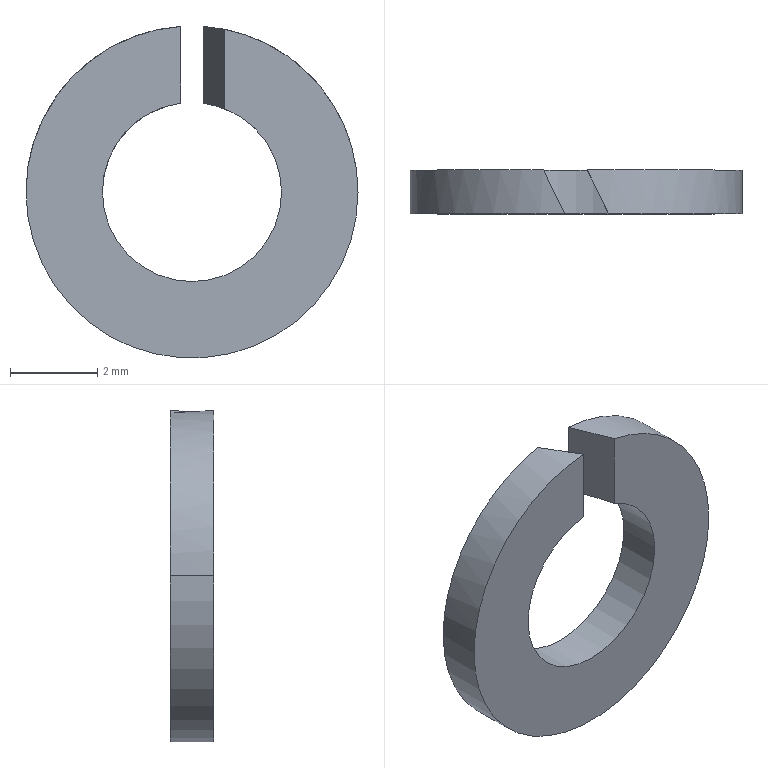Part | STEP file | ZZ24-M4-8 | 1 solid | 10 faces | box 7.6 x 1 x 7.591 mm | volume 30.4 mm3 | cylinder 6 | plane 4 | commonest cylinder face diameters 4.1 x3 7.6 x3
STEP:
#1=CARTESIAN_POINT('',(0.,0.,0.));
#2=DIRECTION('',(0.,0.,1.));
#3=DIRECTION('',(1.,0.,0.));
#4=AXIS2_PLACEMENT_3D('',#1,#2,#3);
#5=CARTESIAN_POINT('',(0.7439,0.,1.91));
#6=VERTEX_POINT('',#5);
#7=CARTESIAN_POINT('',(0.2561,1.,2.034));
#8=VERTEX_POINT('',#7);
#9=CARTESIAN_POINT('',(0.7439,0.,1.91));
#10=CARTESIAN_POINT('',(0.5868,0.3221,1.971));
#11=CARTESIAN_POINT('',(0.4234,0.6571,2.013));
#12=CARTESIAN_POINT('',(0.2561,1.,2.034));
#13=(BOUNDED_CURVE()B_SPLINE_CURVE(3,(#9,#10,#11,#12),.UNSPECIFIED.,.F.,.F.)B_SPLINE_CURVE_WITH_KNOTS((4,4),(1.199,1.446),.PIECEWISE_BEZIER_KNOTS.)CURVE()GEOMETRIC_REPRESENTATION_ITEM()RATIONAL_B_SPLINE_CURVE((1.,0.995,0.995,1.))REPRESENTATION_ITEM(''));
#14=CARTESIAN_POINT('',(0.,1.,0.));
#15=DIRECTION('',(0.,-1.,0.));
#16=DIRECTION('',(-1.,0.,0.001512));
#17=AXIS2_PLACEMENT_3D('',#14,#15,#16);
#18=CYLINDRICAL_SURFACE('',#17,2.05);
#19=CARTESIAN_POINT('',(4.343,1.));
#20=CARTESIAN_POINT('',(4.346,0.9854));
#21=CARTESIAN_POINT('',(4.354,0.9562));
#22=CARTESIAN_POINT('',(4.365,0.9122));
#23=CARTESIAN_POINT('',(4.376,0.868));
#24=CARTESIAN_POINT('',(4.387,0.8236));
#25=CARTESIAN_POINT('',(4.398,0.779));
#26=CARTESIAN_POINT('',(4.41,0.7342));
#27=CARTESIAN_POINT('',(4.421,0.6892));
#28=CARTESIAN_POINT('',(4.432,0.6441));
#29=CARTESIAN_POINT('',(4.443,0.5988));
#30=CARTESIAN_POINT('',(4.454,0.5534));
#31=CARTESIAN_POINT('',(4.466,0.5078));
#32=CARTESIAN_POINT('',(4.477,0.4621));
#33=CARTESIAN_POINT('',(4.488,0.4163));
#34=CARTESIAN_POINT('',(4.499,0.3704));
#35=CARTESIAN_POINT('',(4.51,0.3244));
#36=CARTESIAN_POINT('',(4.522,0.2782));
#37=CARTESIAN_POINT('',(4.533,0.232));
#38=CARTESIAN_POINT('',(4.544,0.1858));
#39=CARTESIAN_POINT('',(4.555,0.1394));
#40=CARTESIAN_POINT('',(4.566,0.09298));
#41=CARTESIAN_POINT('',(4.577,0.04651));
#42=CARTESIAN_POINT('',(4.585,0.01551));
#43=CARTESIAN_POINT('',(4.589,0.));
#44=B_SPLINE_CURVE_WITH_KNOTS('',3,(#19,#20,#21,#22,#23,#24,#25,#26,#27,#28,#29,#30,#31,#32,#33,#34,#35,#36,#37,#38,#39,#40,#41,#42,#43),.UNSPECIFIED.,.F.,.F.,(4,1,1,1,1,1,1,1,1,1,1,1,1,1,1,1,1,1,1,1,1,1,4),(1.199,1.211,1.222,1.233,1.244,1.255,1.267,1.278,1.289,1.3,1.311,1.322,1.334,1.345,1.356,1.367,1.378,1.39,1.401,1.412,1.423,1.434,1.446),.QUASI_UNIFORM_KNOTS.);
#45=(GEOMETRIC_REPRESENTATION_CONTEXT(2)PARAMETRIC_REPRESENTATION_CONTEXT()REPRESENTATION_CONTEXT('',''));
#46=DEFINITIONAL_REPRESENTATION('',(#44),#45);
#47=PCURVE('',#18,#46);
#48=CARTESIAN_POINT('',(0.7439,0.,3.8));
#49=DIRECTION('',(-0.8988,-0.4384,0.));
#50=DIRECTION('',(0.4384,-0.8988,0.));
#51=AXIS2_PLACEMENT_3D('',#48,#49,#50);
#52=PLANE('',#51);
#53=CARTESIAN_POINT('',(0.,-1.89));
#54=CARTESIAN_POINT('',(-0.3583,-1.829));
#55=CARTESIAN_POINT('',(-0.7311,-1.787));
#56=CARTESIAN_POINT('',(-1.113,-1.766));
#57=(BOUNDED_CURVE()B_SPLINE_CURVE(3,(#53,#54,#55,#56),.UNSPECIFIED.,.F.,.F.)B_SPLINE_CURVE_WITH_KNOTS((4,4),(1.199,1.446),.PIECEWISE_BEZIER_KNOTS.)CURVE()GEOMETRIC_REPRESENTATION_ITEM()RATIONAL_B_SPLINE_CURVE((1.,0.995,0.995,1.))REPRESENTATION_ITEM(''));
#58=(GEOMETRIC_REPRESENTATION_CONTEXT(2)PARAMETRIC_REPRESENTATION_CONTEXT()REPRESENTATION_CONTEXT('',''));
#59=DEFINITIONAL_REPRESENTATION('',(#57),#58);
#60=PCURVE('',#52,#59);
#61=SURFACE_CURVE('',#13,(#47,#60),.PCURVE_S1.);
#62=EDGE_CURVE('',#6,#8,#61,.T.);
#63=ORIENTED_EDGE('',*,*,#62,.F.);
#64=CARTESIAN_POINT('',(2.05,0.,-0.0031));
#65=VERTEX_POINT('',#64);
#66=CARTESIAN_POINT('',(0.,0.,0.));
#67=DIRECTION('',(0.,1.,0.));
#68=DIRECTION('',(1.,0.,-0.001512));
#69=AXIS2_PLACEMENT_3D('',#66,#67,#68);
#70=CIRCLE('',#69,2.05);
#71=CARTESIAN_POINT('',(9.425,1.));
#72=DIRECTION('',(-1.,0.));
#73=VECTOR('',#72,1.);
#74=LINE('',#71,#73);
#75=(GEOMETRIC_REPRESENTATION_CONTEXT(2)PARAMETRIC_REPRESENTATION_CONTEXT()REPRESENTATION_CONTEXT('',''));
#76=DEFINITIONAL_REPRESENTATION('',(#74),#75);
#77=PCURVE('',#18,#76);
#78=CARTESIAN_POINT('',(0.,0.,0.));
#79=DIRECTION('',(0.,-1.,0.));
#80=DIRECTION('',(-1.,0.,0.001512));
#81=AXIS2_PLACEMENT_3D('',#78,#79,#80);
#82=PLANE('',#81);
#83=CARTESIAN_POINT('',(-2.05,0.));
#84=CARTESIAN_POINT('',(-2.05,3.551));
#85=CARTESIAN_POINT('',(1.025,1.775));
#86=CARTESIAN_POINT('',(4.1,0.));
#87=CARTESIAN_POINT('',(1.025,-1.775));
#88=CARTESIAN_POINT('',(-2.05,-3.551));
#89=CARTESIAN_POINT('',(-2.05,0.));
#90=(BOUNDED_CURVE()B_SPLINE_CURVE(2,(#83,#84,#85,#86,#87,#88,#89),.UNSPECIFIED.,.T.,.F.)B_SPLINE_CURVE_WITH_KNOTS((1,2,2,2,2,1),(-2.094,0.,2.094,4.189,6.283,8.378),.UNSPECIFIED.)CURVE()GEOMETRIC_REPRESENTATION_ITEM()RATIONAL_B_SPLINE_CURVE((1.,0.5,1.,0.5,1.,0.5,1.))REPRESENTATION_ITEM(''));
#91=(GEOMETRIC_REPRESENTATION_CONTEXT(2)PARAMETRIC_REPRESENTATION_CONTEXT()REPRESENTATION_CONTEXT('',''));
#92=DEFINITIONAL_REPRESENTATION('',(#90),#91);
#93=PCURVE('',#82,#92);
#94=SURFACE_CURVE('',#70,(#77,#93),.PCURVE_S1.);
#95=EDGE_CURVE('',#6,#65,#94,.T.);
#96=ORIENTED_EDGE('',*,*,#95,.T.);
#97=CARTESIAN_POINT('',(2.05,1.,-0.0031));
#98=VERTEX_POINT('',#97);
#99=CARTESIAN_POINT('',(2.05,1.,-0.0031));
#100=DIRECTION('',(0.,-1.,0.));
#101=VECTOR('',#100,1.);
#102=LINE('',#99,#101);
#103=CARTESIAN_POINT('',(3.142,0.));
#104=DIRECTION('',(0.,1.));
#105=VECTOR('',#104,1.);
#106=LINE('',#103,#105);
#107=(GEOMETRIC_REPRESENTATION_CONTEXT(2)PARAMETRIC_REPRESENTATION_CONTEXT()REPRESENTATION_CONTEXT('',''));
#108=DEFINITIONAL_REPRESENTATION('',(#106),#107);
#109=PCURVE('',#18,#108);
#110=CARTESIAN_POINT('',(0.,1.,0.));
#111=DIRECTION('',(0.,-1.,0.));
#112=DIRECTION('',(-1.,0.,0.001512));
#113=AXIS2_PLACEMENT_3D('',#110,#111,#112);
#114=CYLINDRICAL_SURFACE('',#113,2.05);
#115=CARTESIAN_POINT('',(3.142,0.));
#116=DIRECTION('',(0.,1.));
#117=VECTOR('',#116,1.);
#118=LINE('',#115,#117);
#119=(GEOMETRIC_REPRESENTATION_CONTEXT(2)PARAMETRIC_REPRESENTATION_CONTEXT()REPRESENTATION_CONTEXT('',''));
#120=DEFINITIONAL_REPRESENTATION('',(#118),#119);
#121=PCURVE('',#114,#120);
#122=SURFACE_CURVE('',#102,(#109,#121),.PCURVE_S1.);
#123=EDGE_CURVE('',#98,#65,#122,.T.);
#124=ORIENTED_EDGE('',*,*,#123,.F.);
#125=CARTESIAN_POINT('',(0.,1.,0.));
#126=DIRECTION('',(0.,-1.,0.));
#127=DIRECTION('',(-1.,0.,0.001512));
#128=AXIS2_PLACEMENT_3D('',#125,#126,#127);
#129=CIRCLE('',#128,2.05);
#130=CARTESIAN_POINT('',(0.,0.));
#131=DIRECTION('',(1.,0.));
#132=VECTOR('',#131,1.);
#133=LINE('',#130,#132);
#134=(GEOMETRIC_REPRESENTATION_CONTEXT(2)PARAMETRIC_REPRESENTATION_CONTEXT()REPRESENTATION_CONTEXT('',''));
#135=DEFINITIONAL_REPRESENTATION('',(#133),#134);
#136=PCURVE('',#18,#135);
#137=CARTESIAN_POINT('',(0.,1.,0.));
#138=DIRECTION('',(0.,1.,0.));
#139=DIRECTION('',(1.,0.,-0.001512));
#140=AXIS2_PLACEMENT_3D('',#137,#138,#139);
#141=PLANE('',#140);
#142=CARTESIAN_POINT('',(-2.05,0.));
#143=CARTESIAN_POINT('',(-2.05,3.551));
#144=CARTESIAN_POINT('',(1.025,1.775));
#145=CARTESIAN_POINT('',(4.1,0.));
#146=CARTESIAN_POINT('',(1.025,-1.775));
#147=CARTESIAN_POINT('',(-2.05,-3.551));
#148=CARTESIAN_POINT('',(-2.05,0.));
#149=(BOUNDED_CURVE()B_SPLINE_CURVE(2,(#142,#143,#144,#145,#146,#147,#148),.UNSPECIFIED.,.T.,.F.)B_SPLINE_CURVE_WITH_KNOTS((1,2,2,2,2,1),(-2.094,0.,2.094,4.189,6.283,8.378),.UNSPECIFIED.)CURVE()GEOMETRIC_REPRESENTATION_ITEM()RATIONAL_B_SPLINE_CURVE((1.,0.5,1.,0.5,1.,0.5,1.))REPRESENTATION_ITEM(''));
#150=(GEOMETRIC_REPRESENTATION_CONTEXT(2)PARAMETRIC_REPRESENTATION_CONTEXT()REPRESENTATION_CONTEXT('',''));
#151=DEFINITIONAL_REPRESENTATION('',(#149),#150);
#152=PCURVE('',#141,#151);
#153=SURFACE_CURVE('',#129,(#136,#152),.PCURVE_S1.);
#154=EDGE_CURVE('',#98,#8,#153,.T.);
#155=ORIENTED_EDGE('',*,*,#154,.T.);
#156=EDGE_LOOP('',(#63,#96,#124,#155));
#157=FACE_BOUND('',#156,.F.);
#158=ADVANCED_FACE('',(#157),#18,.F.);
#159=CARTESIAN_POINT('',(-2.05,0.,0.0031));
#160=VERTEX_POINT('',#159);
#161=CARTESIAN_POINT('',(0.,0.,0.));
#162=DIRECTION('',(0.,1.,0.));
#163=DIRECTION('',(1.,0.,-0.001512));
#164=AXIS2_PLACEMENT_3D('',#161,#162,#163);
#165=CIRCLE('',#164,2.05);
#166=CARTESIAN_POINT('',(3.142,1.));
#167=DIRECTION('',(-1.,0.));
#168=VECTOR('',#167,1.);
#169=LINE('',#166,#168);
#170=(GEOMETRIC_REPRESENTATION_CONTEXT(2)PARAMETRIC_REPRESENTATION_CONTEXT()REPRESENTATION_CONTEXT('',''));
#171=DEFINITIONAL_REPRESENTATION('',(#169),#170);
#172=PCURVE('',#114,#171);
#173=CARTESIAN_POINT('',(-2.05,0.));
#174=CARTESIAN_POINT('',(-2.05,3.551));
#175=CARTESIAN_POINT('',(1.025,1.775));
#176=CARTESIAN_POINT('',(4.1,0.));
#177=CARTESIAN_POINT('',(1.025,-1.775));
#178=CARTESIAN_POINT('',(-2.05,-3.551));
#179=CARTESIAN_POINT('',(-2.05,0.));
#180=(BOUNDED_CURVE()B_SPLINE_CURVE(2,(#173,#174,#175,#176,#177,#178,#179),.UNSPECIFIED.,.T.,.F.)B_SPLINE_CURVE_WITH_KNOTS((1,2,2,2,2,1),(-2.094,0.,2.094,4.189,6.283,8.378),.UNSPECIFIED.)CURVE()GEOMETRIC_REPRESENTATION_ITEM()RATIONAL_B_SPLINE_CURVE((1.,0.5,1.,0.5,1.,0.5,1.))REPRESENTATION_ITEM(''));
#181=(GEOMETRIC_REPRESENTATION_CONTEXT(2)PARAMETRIC_REPRESENTATION_CONTEXT()REPRESENTATION_CONTEXT('',''));
#182=DEFINITIONAL_REPRESENTATION('',(#180),#181);
#183=PCURVE('',#82,#182);
#184=SURFACE_CURVE('',#165,(#172,#183),.PCURVE_S1.);
#185=EDGE_CURVE('',#65,#160,#184,.T.);
#186=ORIENTED_EDGE('',*,*,#185,.T.);
#187=CARTESIAN_POINT('',(-2.05,1.,0.0031));
#188=VERTEX_POINT('',#187);
#189=CARTESIAN_POINT('',(-2.05,1.,0.0031));
#190=DIRECTION('',(0.,-1.,0.));
#191=VECTOR('',#190,1.);
#192=LINE('',#189,#191);
#193=CARTESIAN_POINT('',(0.,0.));
#194=DIRECTION('',(0.,1.));
#195=VECTOR('',#194,1.);
#196=LINE('',#193,#195);
#197=(GEOMETRIC_REPRESENTATION_CONTEXT(2)PARAMETRIC_REPRESENTATION_CONTEXT()REPRESENTATION_CONTEXT('',''));
#198=DEFINITIONAL_REPRESENTATION('',(#196),#197);
#199=PCURVE('',#114,#198);
#200=CARTESIAN_POINT('',(0.,1.,0.));
#201=DIRECTION('',(0.,-1.,0.));
#202=DIRECTION('',(-1.,0.,0.001512));
#203=AXIS2_PLACEMENT_3D('',#200,#201,#202);
#204=CYLINDRICAL_SURFACE('',#203,2.05);
#205=CARTESIAN_POINT('',(6.283,0.));
#206=DIRECTION('',(0.,1.));
#207=VECTOR('',#206,1.);
#208=LINE('',#205,#207);
#209=(GEOMETRIC_REPRESENTATION_CONTEXT(2)PARAMETRIC_REPRESENTATION_CONTEXT()REPRESENTATION_CONTEXT('',''));
#210=DEFINITIONAL_REPRESENTATION('',(#208),#209);
#211=PCURVE('',#204,#210);
#212=SURFACE_CURVE('',#192,(#199,#211),.PCURVE_S1.);
#213=EDGE_CURVE('',#188,#160,#212,.T.);
#214=ORIENTED_EDGE('',*,*,#213,.F.);
#215=CARTESIAN_POINT('',(0.,1.,0.));
#216=DIRECTION('',(0.,-1.,0.));
#217=DIRECTION('',(-1.,0.,0.001512));
#218=AXIS2_PLACEMENT_3D('',#215,#216,#217);
#219=CIRCLE('',#218,2.05);
#220=CARTESIAN_POINT('',(0.,0.));
#221=DIRECTION('',(1.,0.));
#222=VECTOR('',#221,1.);
#223=LINE('',#220,#222);
#224=(GEOMETRIC_REPRESENTATION_CONTEXT(2)PARAMETRIC_REPRESENTATION_CONTEXT()REPRESENTATION_CONTEXT('',''));
#225=DEFINITIONAL_REPRESENTATION('',(#223),#224);
#226=PCURVE('',#114,#225);
#227=CARTESIAN_POINT('',(-2.05,0.));
#228=CARTESIAN_POINT('',(-2.05,3.551));
#229=CARTESIAN_POINT('',(1.025,1.775));
#230=CARTESIAN_POINT('',(4.1,0.));
#231=CARTESIAN_POINT('',(1.025,-1.775));
#232=CARTESIAN_POINT('',(-2.05,-3.551));
#233=CARTESIAN_POINT('',(-2.05,0.));
#234=(BOUNDED_CURVE()B_SPLINE_CURVE(2,(#227,#228,#229,#230,#231,#232,#233),.UNSPECIFIED.,.T.,.F.)B_SPLINE_CURVE_WITH_KNOTS((1,2,2,2,2,1),(-2.094,0.,2.094,4.189,6.283,8.378),.UNSPECIFIED.)CURVE()GEOMETRIC_REPRESENTATION_ITEM()RATIONAL_B_SPLINE_CURVE((1.,0.5,1.,0.5,1.,0.5,1.))REPRESENTATION_ITEM(''));
#235=(GEOMETRIC_REPRESENTATION_CONTEXT(2)PARAMETRIC_REPRESENTATION_CONTEXT()REPRESENTATION_CONTEXT('',''));
#236=DEFINITIONAL_REPRESENTATION('',(#234),#235);
#237=PCURVE('',#141,#236);
#238=SURFACE_CURVE('',#219,(#226,#237),.PCURVE_S1.);
#239=EDGE_CURVE('',#188,#98,#238,.T.);
#240=ORIENTED_EDGE('',*,*,#239,.T.);
#241=ORIENTED_EDGE('',*,*,#123,.T.);
#242=EDGE_LOOP('',(#186,#214,#240,#241));
#243=FACE_BOUND('',#242,.F.);
#244=ADVANCED_FACE('',(#243),#114,.F.);
#245=CARTESIAN_POINT('',(-3.8,1.,0.005747));
#246=VERTEX_POINT('',#245);
#247=CARTESIAN_POINT('',(3.8,1.,-0.005747));
#248=VERTEX_POINT('',#247);
#249=CARTESIAN_POINT('',(0.,1.,0.));
#250=DIRECTION('',(0.,-1.,0.));
#251=DIRECTION('',(-1.,0.,0.001512));
#252=AXIS2_PLACEMENT_3D('',#249,#250,#251);
#253=CIRCLE('',#252,3.8);
#254=CARTESIAN_POINT('',(0.,1.,0.));
#255=DIRECTION('',(0.,-1.,0.));
#256=DIRECTION('',(-1.,0.,0.001512));
#257=AXIS2_PLACEMENT_3D('',#254,#255,#256);
#258=CYLINDRICAL_SURFACE('',#257,3.8);
#259=CARTESIAN_POINT('',(0.,0.));
#260=DIRECTION('',(1.,0.));
#261=VECTOR('',#260,1.);
#262=LINE('',#259,#261);
#263=(GEOMETRIC_REPRESENTATION_CONTEXT(2)PARAMETRIC_REPRESENTATION_CONTEXT()REPRESENTATION_CONTEXT('',''));
#264=DEFINITIONAL_REPRESENTATION('',(#262),#263);
#265=PCURVE('',#258,#264);
#266=CARTESIAN_POINT('',(-3.8,0.));
#267=CARTESIAN_POINT('',(-3.8,6.582));
#268=CARTESIAN_POINT('',(1.9,3.291));
#269=CARTESIAN_POINT('',(7.6,0.));
#270=CARTESIAN_POINT('',(1.9,-3.291));
#271=CARTESIAN_POINT('',(-3.8,-6.582));
#272=CARTESIAN_POINT('',(-3.8,0.));
#273=(BOUNDED_CURVE()B_SPLINE_CURVE(2,(#266,#267,#268,#269,#270,#271,#272),.UNSPECIFIED.,.T.,.F.)B_SPLINE_CURVE_WITH_KNOTS((1,2,2,2,2,1),(-2.094,0.,2.094,4.189,6.283,8.378),.UNSPECIFIED.)CURVE()GEOMETRIC_REPRESENTATION_ITEM()RATIONAL_B_SPLINE_CURVE((1.,0.5,1.,0.5,1.,0.5,1.))REPRESENTATION_ITEM(''));
#274=(GEOMETRIC_REPRESENTATION_CONTEXT(2)PARAMETRIC_REPRESENTATION_CONTEXT()REPRESENTATION_CONTEXT('',''));
#275=DEFINITIONAL_REPRESENTATION('',(#273),#274);
#276=PCURVE('',#141,#275);
#277=SURFACE_CURVE('',#253,(#265,#276),.PCURVE_S1.);
#278=EDGE_CURVE('',#246,#248,#277,.T.);
#279=ORIENTED_EDGE('',*,*,#278,.T.);
#280=CARTESIAN_POINT('',(3.8,0.,-0.005747));
#281=VERTEX_POINT('',#280);
#282=CARTESIAN_POINT('',(3.8,1.,-0.005747));
#283=DIRECTION('',(0.,-1.,0.));
#284=VECTOR('',#283,1.);
#285=LINE('',#282,#284);
#286=CARTESIAN_POINT('',(3.142,0.));
#287=DIRECTION('',(0.,1.));
#288=VECTOR('',#287,1.);
#289=LINE('',#286,#288);
#290=(GEOMETRIC_REPRESENTATION_CONTEXT(2)PARAMETRIC_REPRESENTATION_CONTEXT()REPRESENTATION_CONTEXT('',''));
#291=DEFINITIONAL_REPRESENTATION('',(#289),#290);
#292=PCURVE('',#258,#291);
#293=CARTESIAN_POINT('',(0.,1.,0.));
#294=DIRECTION('',(0.,-1.,0.));
#295=DIRECTION('',(-1.,0.,0.001512));
#296=AXIS2_PLACEMENT_3D('',#293,#294,#295);
#297=CYLINDRICAL_SURFACE('',#296,3.8);
#298=CARTESIAN_POINT('',(3.142,0.));
#299=DIRECTION('',(0.,1.));
#300=VECTOR('',#299,1.);
#301=LINE('',#298,#300);
#302=(GEOMETRIC_REPRESENTATION_CONTEXT(2)PARAMETRIC_REPRESENTATION_CONTEXT()REPRESENTATION_CONTEXT('',''));
#303=DEFINITIONAL_REPRESENTATION('',(#301),#302);
#304=PCURVE('',#297,#303);
#305=SURFACE_CURVE('',#285,(#292,#304),.PCURVE_S1.);
#306=EDGE_CURVE('',#248,#281,#305,.T.);
#307=ORIENTED_EDGE('',*,*,#306,.T.);
#308=CARTESIAN_POINT('',(-3.8,0.,0.005747));
#309=VERTEX_POINT('',#308);
#310=CARTESIAN_POINT('',(0.,0.,0.));
#311=DIRECTION('',(0.,1.,0.));
#312=DIRECTION('',(1.,0.,-0.001512));
#313=AXIS2_PLACEMENT_3D('',#310,#311,#312);
#314=CIRCLE('',#313,3.8);
#315=CARTESIAN_POINT('',(3.142,1.));
#316=DIRECTION('',(-1.,0.));
#317=VECTOR('',#316,1.);
#318=LINE('',#315,#317);
#319=(GEOMETRIC_REPRESENTATION_CONTEXT(2)PARAMETRIC_REPRESENTATION_CONTEXT()REPRESENTATION_CONTEXT('',''));
#320=DEFINITIONAL_REPRESENTATION('',(#318),#319);
#321=PCURVE('',#258,#320);
#322=CARTESIAN_POINT('',(-3.8,0.));
#323=CARTESIAN_POINT('',(-3.8,6.582));
#324=CARTESIAN_POINT('',(1.9,3.291));
#325=CARTESIAN_POINT('',(7.6,0.));
#326=CARTESIAN_POINT('',(1.9,-3.291));
#327=CARTESIAN_POINT('',(-3.8,-6.582));
#328=CARTESIAN_POINT('',(-3.8,0.));
#329=(BOUNDED_CURVE()B_SPLINE_CURVE(2,(#322,#323,#324,#325,#326,#327,#328),.UNSPECIFIED.,.T.,.F.)B_SPLINE_CURVE_WITH_KNOTS((1,2,2,2,2,1),(-2.094,0.,2.094,4.189,6.283,8.378),.UNSPECIFIED.)CURVE()GEOMETRIC_REPRESENTATION_ITEM()RATIONAL_B_SPLINE_CURVE((1.,0.5,1.,0.5,1.,0.5,1.))REPRESENTATION_ITEM(''));
#330=(GEOMETRIC_REPRESENTATION_CONTEXT(2)PARAMETRIC_REPRESENTATION_CONTEXT()REPRESENTATION_CONTEXT('',''));
#331=DEFINITIONAL_REPRESENTATION('',(#329),#330);
#332=PCURVE('',#82,#331);
#333=SURFACE_CURVE('',#314,(#321,#332),.PCURVE_S1.);
#334=EDGE_CURVE('',#281,#309,#333,.T.);
#335=ORIENTED_EDGE('',*,*,#334,.T.);
#336=CARTESIAN_POINT('',(-3.8,1.,0.005747));
#337=DIRECTION('',(0.,-1.,0.));
#338=VECTOR('',#337,1.);
#339=LINE('',#336,#338);
#340=CARTESIAN_POINT('',(0.,0.));
#341=DIRECTION('',(0.,1.));
#342=VECTOR('',#341,1.);
#343=LINE('',#340,#342);
#344=(GEOMETRIC_REPRESENTATION_CONTEXT(2)PARAMETRIC_REPRESENTATION_CONTEXT()REPRESENTATION_CONTEXT('',''));
#345=DEFINITIONAL_REPRESENTATION('',(#343),#344);
#346=PCURVE('',#258,#345);
#347=CARTESIAN_POINT('',(0.,1.,0.));
#348=DIRECTION('',(0.,-1.,0.));
#349=DIRECTION('',(-1.,0.,0.001512));
#350=AXIS2_PLACEMENT_3D('',#347,#348,#349);
#351=CYLINDRICAL_SURFACE('',#350,3.8);
#352=CARTESIAN_POINT('',(6.283,0.));
#353=DIRECTION('',(0.,1.));
#354=VECTOR('',#353,1.);
#355=LINE('',#352,#354);
#356=(GEOMETRIC_REPRESENTATION_CONTEXT(2)PARAMETRIC_REPRESENTATION_CONTEXT()REPRESENTATION_CONTEXT('',''));
#357=DEFINITIONAL_REPRESENTATION('',(#355),#356);
#358=PCURVE('',#351,#357);
#359=SURFACE_CURVE('',#339,(#346,#358),.PCURVE_S1.);
#360=EDGE_CURVE('',#246,#309,#359,.T.);
#361=ORIENTED_EDGE('',*,*,#360,.F.);
#362=EDGE_LOOP('',(#279,#307,#335,#361));
#363=FACE_BOUND('',#362,.T.);
#364=ADVANCED_FACE('',(#363),#258,.T.);
#365=CARTESIAN_POINT('',(-0.7439,1.,3.726));
#366=VERTEX_POINT('',#365);
#367=CARTESIAN_POINT('',(0.,1.,0.));
#368=DIRECTION('',(0.,-1.,0.));
#369=DIRECTION('',(-1.,0.,0.001512));
#370=AXIS2_PLACEMENT_3D('',#367,#368,#369);
#371=CIRCLE('',#370,3.8);
#372=CARTESIAN_POINT('',(0.,0.));
#373=DIRECTION('',(1.,0.));
#374=VECTOR('',#373,1.);
#375=LINE('',#372,#374);
#376=(GEOMETRIC_REPRESENTATION_CONTEXT(2)PARAMETRIC_REPRESENTATION_CONTEXT()REPRESENTATION_CONTEXT('',''));
#377=DEFINITIONAL_REPRESENTATION('',(#375),#376);
#378=PCURVE('',#351,#377);
#379=CARTESIAN_POINT('',(-3.8,0.));
#380=CARTESIAN_POINT('',(-3.8,6.582));
#381=CARTESIAN_POINT('',(1.9,3.291));
#382=CARTESIAN_POINT('',(7.6,0.));
#383=CARTESIAN_POINT('',(1.9,-3.291));
#384=CARTESIAN_POINT('',(-3.8,-6.582));
#385=CARTESIAN_POINT('',(-3.8,0.));
#386=(BOUNDED_CURVE()B_SPLINE_CURVE(2,(#379,#380,#381,#382,#383,#384,#385),.UNSPECIFIED.,.T.,.F.)B_SPLINE_CURVE_WITH_KNOTS((1,2,2,2,2,1),(-2.094,0.,2.094,4.189,6.283,8.378),.UNSPECIFIED.)CURVE()GEOMETRIC_REPRESENTATION_ITEM()RATIONAL_B_SPLINE_CURVE((1.,0.5,1.,0.5,1.,0.5,1.))REPRESENTATION_ITEM(''));
#387=(GEOMETRIC_REPRESENTATION_CONTEXT(2)PARAMETRIC_REPRESENTATION_CONTEXT()REPRESENTATION_CONTEXT('',''));
#388=DEFINITIONAL_REPRESENTATION('',(#386),#387);
#389=PCURVE('',#141,#388);
#390=SURFACE_CURVE('',#371,(#378,#389),.PCURVE_S1.);
#391=EDGE_CURVE('',#366,#246,#390,.T.);
#392=ORIENTED_EDGE('',*,*,#391,.T.);
#393=ORIENTED_EDGE('',*,*,#360,.T.);
#394=CARTESIAN_POINT('',(-0.2561,0.,3.791));
#395=VERTEX_POINT('',#394);
#396=CARTESIAN_POINT('',(0.,0.,0.));
#397=DIRECTION('',(0.,1.,0.));
#398=DIRECTION('',(1.,0.,-0.001512));
#399=AXIS2_PLACEMENT_3D('',#396,#397,#398);
#400=CIRCLE('',#399,3.8);
#401=CARTESIAN_POINT('',(9.425,1.));
#402=DIRECTION('',(-1.,0.));
#403=VECTOR('',#402,1.);
#404=LINE('',#401,#403);
#405=(GEOMETRIC_REPRESENTATION_CONTEXT(2)PARAMETRIC_REPRESENTATION_CONTEXT()REPRESENTATION_CONTEXT('',''));
#406=DEFINITIONAL_REPRESENTATION('',(#404),#405);
#407=PCURVE('',#351,#406);
#408=CARTESIAN_POINT('',(-3.8,0.));
#409=CARTESIAN_POINT('',(-3.8,6.582));
#410=CARTESIAN_POINT('',(1.9,3.291));
#411=CARTESIAN_POINT('',(7.6,0.));
#412=CARTESIAN_POINT('',(1.9,-3.291));
#413=CARTESIAN_POINT('',(-3.8,-6.582));
#414=CARTESIAN_POINT('',(-3.8,0.));
#415=(BOUNDED_CURVE()B_SPLINE_CURVE(2,(#408,#409,#410,#411,#412,#413,#414),.UNSPECIFIED.,.T.,.F.)B_SPLINE_CURVE_WITH_KNOTS((1,2,2,2,2,1),(-2.094,0.,2.094,4.189,6.283,8.378),.UNSPECIFIED.)CURVE()GEOMETRIC_REPRESENTATION_ITEM()RATIONAL_B_SPLINE_CURVE((1.,0.5,1.,0.5,1.,0.5,1.))REPRESENTATION_ITEM(''));
#416=(GEOMETRIC_REPRESENTATION_CONTEXT(2)PARAMETRIC_REPRESENTATION_CONTEXT()REPRESENTATION_CONTEXT('',''));
#417=DEFINITIONAL_REPRESENTATION('',(#415),#416);
#418=PCURVE('',#82,#417);
#419=SURFACE_CURVE('',#400,(#407,#418),.PCURVE_S1.);
#420=EDGE_CURVE('',#309,#395,#419,.T.);
#421=ORIENTED_EDGE('',*,*,#420,.T.);
#422=CARTESIAN_POINT('',(-0.2561,0.,3.791));
#423=CARTESIAN_POINT('',(-0.42,0.336,3.78));
#424=CARTESIAN_POINT('',(-0.5828,0.6698,3.759));
#425=CARTESIAN_POINT('',(-0.7439,1.,3.726));
#426=(BOUNDED_CURVE()B_SPLINE_CURVE(3,(#422,#423,#424,#425),.UNSPECIFIED.,.F.,.F.)B_SPLINE_CURVE_WITH_KNOTS((4,4),(1.638,1.768),.PIECEWISE_BEZIER_KNOTS.)CURVE()GEOMETRIC_REPRESENTATION_ITEM()RATIONAL_B_SPLINE_CURVE((1.,0.9986,0.9986,1.))REPRESENTATION_ITEM(''));
#427=CARTESIAN_POINT('',(4.781,1.));
#428=CARTESIAN_POINT('',(4.783,0.9847));
#429=CARTESIAN_POINT('',(4.787,0.9543));
#430=CARTESIAN_POINT('',(4.793,0.9085));
#431=CARTESIAN_POINT('',(4.799,0.8628));
#432=CARTESIAN_POINT('',(4.805,0.8171));
#433=CARTESIAN_POINT('',(4.811,0.7714));
#434=CARTESIAN_POINT('',(4.817,0.7257));
#435=CARTESIAN_POINT('',(4.823,0.6801));
#436=CARTESIAN_POINT('',(4.828,0.6345));
#437=CARTESIAN_POINT('',(4.834,0.5889));
#438=CARTESIAN_POINT('',(4.84,0.5434));
#439=CARTESIAN_POINT('',(4.846,0.4978));
#440=CARTESIAN_POINT('',(4.852,0.4524));
#441=CARTESIAN_POINT('',(4.858,0.4069));
#442=CARTESIAN_POINT('',(4.864,0.3615));
#443=CARTESIAN_POINT('',(4.87,0.3161));
#444=CARTESIAN_POINT('',(4.876,0.2708));
#445=CARTESIAN_POINT('',(4.881,0.2255));
#446=CARTESIAN_POINT('',(4.887,0.1803));
#447=CARTESIAN_POINT('',(4.893,0.1352));
#448=CARTESIAN_POINT('',(4.899,0.09005));
#449=CARTESIAN_POINT('',(4.905,0.04499));
#450=CARTESIAN_POINT('',(4.909,0.01499));
#451=CARTESIAN_POINT('',(4.911,0.));
#452=B_SPLINE_CURVE_WITH_KNOTS('',3,(#427,#428,#429,#430,#431,#432,#433,#434,#435,#436,#437,#438,#439,#440,#441,#442,#443,#444,#445,#446,#447,#448,#449,#450,#451),.UNSPECIFIED.,.F.,.F.,(4,1,1,1,1,1,1,1,1,1,1,1,1,1,1,1,1,1,1,1,1,1,4),(1.638,1.644,1.65,1.656,1.662,1.668,1.674,1.679,1.685,1.691,1.697,1.703,1.709,1.715,1.721,1.727,1.732,1.738,1.744,1.75,1.756,1.762,1.768),.QUASI_UNIFORM_KNOTS.);
#453=(GEOMETRIC_REPRESENTATION_CONTEXT(2)PARAMETRIC_REPRESENTATION_CONTEXT()REPRESENTATION_CONTEXT('',''));
#454=DEFINITIONAL_REPRESENTATION('',(#452),#453);
#455=PCURVE('',#351,#454);
#456=CARTESIAN_POINT('',(-0.7439,1.,3.8));
#457=DIRECTION('',(0.8988,0.4384,0.));
#458=DIRECTION('',(-0.4384,0.8988,0.));
#459=AXIS2_PLACEMENT_3D('',#456,#457,#458);
#460=PLANE('',#459);
#461=CARTESIAN_POINT('',(-1.113,-0.008642));
#462=CARTESIAN_POINT('',(-0.7388,-0.01971));
#463=CARTESIAN_POINT('',(-0.3674,-0.04137));
#464=CARTESIAN_POINT('',(0.,-0.07352));
#465=(BOUNDED_CURVE()B_SPLINE_CURVE(3,(#461,#462,#463,#464),.UNSPECIFIED.,.F.,.F.)B_SPLINE_CURVE_WITH_KNOTS((4,4),(1.638,1.768),.PIECEWISE_BEZIER_KNOTS.)CURVE()GEOMETRIC_REPRESENTATION_ITEM()RATIONAL_B_SPLINE_CURVE((1.,0.9986,0.9986,1.))REPRESENTATION_ITEM(''));
#466=(GEOMETRIC_REPRESENTATION_CONTEXT(2)PARAMETRIC_REPRESENTATION_CONTEXT()REPRESENTATION_CONTEXT('',''));
#467=DEFINITIONAL_REPRESENTATION('',(#465),#466);
#468=PCURVE('',#460,#467);
#469=SURFACE_CURVE('',#426,(#455,#468),.PCURVE_S1.);
#470=EDGE_CURVE('',#395,#366,#469,.T.);
#471=ORIENTED_EDGE('',*,*,#470,.T.);
#472=EDGE_LOOP('',(#392,#393,#421,#471));
#473=FACE_BOUND('',#472,.T.);
#474=ADVANCED_FACE('',(#473),#351,.T.);
#475=CARTESIAN_POINT('',(-0.2561,0.,2.034));
#476=VERTEX_POINT('',#475);
#477=CARTESIAN_POINT('',(-0.2561,0.,3.8));
#478=DIRECTION('',(0.,0.,-1.));
#479=VECTOR('',#478,1.);
#480=LINE('',#477,#479);
#481=CARTESIAN_POINT('',(0.2619,-3.8));
#482=DIRECTION('',(-0.001512,1.));
#483=VECTOR('',#482,1.);
#484=LINE('',#481,#483);
#485=(GEOMETRIC_REPRESENTATION_CONTEXT(2)PARAMETRIC_REPRESENTATION_CONTEXT()REPRESENTATION_CONTEXT('',''));
#486=DEFINITIONAL_REPRESENTATION('',(#484),#485);
#487=PCURVE('',#82,#486);
#488=CARTESIAN_POINT('',(-1.113,0.));
#489=DIRECTION('',(0.,-1.));
#490=VECTOR('',#489,1.);
#491=LINE('',#488,#490);
#492=(GEOMETRIC_REPRESENTATION_CONTEXT(2)PARAMETRIC_REPRESENTATION_CONTEXT()REPRESENTATION_CONTEXT('',''));
#493=DEFINITIONAL_REPRESENTATION('',(#491),#492);
#494=PCURVE('',#460,#493);
#495=SURFACE_CURVE('',#480,(#487,#494),.PCURVE_S1.);
#496=EDGE_CURVE('',#395,#476,#495,.T.);
#497=ORIENTED_EDGE('',*,*,#496,.F.);
#498=ORIENTED_EDGE('',*,*,#420,.F.);
#499=ORIENTED_EDGE('',*,*,#334,.F.);
#500=CARTESIAN_POINT('',(0.7439,0.,3.726));
#501=VERTEX_POINT('',#500);
#502=CARTESIAN_POINT('',(0.,0.,0.));
#503=DIRECTION('',(0.,1.,0.));
#504=DIRECTION('',(1.,0.,-0.001512));
#505=AXIS2_PLACEMENT_3D('',#502,#503,#504);
#506=CIRCLE('',#505,3.8);
#507=CARTESIAN_POINT('',(-3.8,0.));
#508=CARTESIAN_POINT('',(-3.8,6.582));
#509=CARTESIAN_POINT('',(1.9,3.291));
#510=CARTESIAN_POINT('',(7.6,0.));
#511=CARTESIAN_POINT('',(1.9,-3.291));
#512=CARTESIAN_POINT('',(-3.8,-6.582));
#513=CARTESIAN_POINT('',(-3.8,0.));
#514=(BOUNDED_CURVE()B_SPLINE_CURVE(2,(#507,#508,#509,#510,#511,#512,#513),.UNSPECIFIED.,.T.,.F.)B_SPLINE_CURVE_WITH_KNOTS((1,2,2,2,2,1),(-2.094,0.,2.094,4.189,6.283,8.378),.UNSPECIFIED.)CURVE()GEOMETRIC_REPRESENTATION_ITEM()RATIONAL_B_SPLINE_CURVE((1.,0.5,1.,0.5,1.,0.5,1.))REPRESENTATION_ITEM(''));
#515=(GEOMETRIC_REPRESENTATION_CONTEXT(2)PARAMETRIC_REPRESENTATION_CONTEXT()REPRESENTATION_CONTEXT('',''));
#516=DEFINITIONAL_REPRESENTATION('',(#514),#515);
#517=PCURVE('',#82,#516);
#518=CARTESIAN_POINT('',(9.425,1.));
#519=DIRECTION('',(-1.,0.));
#520=VECTOR('',#519,1.);
#521=LINE('',#518,#520);
#522=(GEOMETRIC_REPRESENTATION_CONTEXT(2)PARAMETRIC_REPRESENTATION_CONTEXT()REPRESENTATION_CONTEXT('',''));
#523=DEFINITIONAL_REPRESENTATION('',(#521),#522);
#524=PCURVE('',#297,#523);
#525=SURFACE_CURVE('',#506,(#517,#524),.PCURVE_S1.);
#526=EDGE_CURVE('',#501,#281,#525,.T.);
#527=ORIENTED_EDGE('',*,*,#526,.F.);
#528=CARTESIAN_POINT('',(0.7439,0.,3.8));
#529=DIRECTION('',(0.,0.,-1.));
#530=VECTOR('',#529,1.);
#531=LINE('',#528,#530);
#532=CARTESIAN_POINT('',(-0.7381,-3.801));
#533=DIRECTION('',(-0.001512,1.));
#534=VECTOR('',#533,1.);
#535=LINE('',#532,#534);
#536=(GEOMETRIC_REPRESENTATION_CONTEXT(2)PARAMETRIC_REPRESENTATION_CONTEXT()REPRESENTATION_CONTEXT('',''));
#537=DEFINITIONAL_REPRESENTATION('',(#535),#536);
#538=PCURVE('',#82,#537);
#539=CARTESIAN_POINT('',(0.,0.));
#540=DIRECTION('',(0.,-1.));
#541=VECTOR('',#540,1.);
#542=LINE('',#539,#541);
#543=(GEOMETRIC_REPRESENTATION_CONTEXT(2)PARAMETRIC_REPRESENTATION_CONTEXT()REPRESENTATION_CONTEXT('',''));
#544=DEFINITIONAL_REPRESENTATION('',(#542),#543);
#545=PCURVE('',#52,#544);
#546=SURFACE_CURVE('',#531,(#538,#545),.PCURVE_S1.);
#547=EDGE_CURVE('',#501,#6,#546,.T.);
#548=ORIENTED_EDGE('',*,*,#547,.T.);
#549=ORIENTED_EDGE('',*,*,#95,.T.);
#550=ORIENTED_EDGE('',*,*,#185,.T.);
#551=CARTESIAN_POINT('',(0.,0.,0.));
#552=DIRECTION('',(0.,1.,0.));
#553=DIRECTION('',(1.,0.,-0.001512));
#554=AXIS2_PLACEMENT_3D('',#551,#552,#553);
#555=CIRCLE('',#554,2.05);
#556=CARTESIAN_POINT('',(-2.05,0.));
#557=CARTESIAN_POINT('',(-2.05,3.551));
#558=CARTESIAN_POINT('',(1.025,1.775));
#559=CARTESIAN_POINT('',(4.1,0.));
#560=CARTESIAN_POINT('',(1.025,-1.775));
#561=CARTESIAN_POINT('',(-2.05,-3.551));
#562=CARTESIAN_POINT('',(-2.05,0.));
#563=(BOUNDED_CURVE()B_SPLINE_CURVE(2,(#556,#557,#558,#559,#560,#561,#562),.UNSPECIFIED.,.T.,.F.)B_SPLINE_CURVE_WITH_KNOTS((1,2,2,2,2,1),(-2.094,0.,2.094,4.189,6.283,8.378),.UNSPECIFIED.)CURVE()GEOMETRIC_REPRESENTATION_ITEM()RATIONAL_B_SPLINE_CURVE((1.,0.5,1.,0.5,1.,0.5,1.))REPRESENTATION_ITEM(''));
#564=(GEOMETRIC_REPRESENTATION_CONTEXT(2)PARAMETRIC_REPRESENTATION_CONTEXT()REPRESENTATION_CONTEXT('',''));
#565=DEFINITIONAL_REPRESENTATION('',(#563),#564);
#566=PCURVE('',#82,#565);
#567=CARTESIAN_POINT('',(9.425,1.));
#568=DIRECTION('',(-1.,0.));
#569=VECTOR('',#568,1.);
#570=LINE('',#567,#569);
#571=(GEOMETRIC_REPRESENTATION_CONTEXT(2)PARAMETRIC_REPRESENTATION_CONTEXT()REPRESENTATION_CONTEXT('',''));
#572=DEFINITIONAL_REPRESENTATION('',(#570),#571);
#573=PCURVE('',#204,#572);
#574=SURFACE_CURVE('',#555,(#566,#573),.PCURVE_S1.);
#575=EDGE_CURVE('',#160,#476,#574,.T.);
#576=ORIENTED_EDGE('',*,*,#575,.T.);
#577=EDGE_LOOP('',(#497,#498,#499,#527,#548,#549,#550,#576));
#578=FACE_BOUND('',#577,.T.);
#579=ADVANCED_FACE('',(#578),#82,.T.);
#580=CARTESIAN_POINT('',(0.2561,1.,3.791));
#581=VERTEX_POINT('',#580);
#582=CARTESIAN_POINT('',(0.2561,1.,3.8));
#583=DIRECTION('',(0.,0.,-1.));
#584=VECTOR('',#583,1.);
#585=LINE('',#582,#584);
#586=CARTESIAN_POINT('',(0.2504,-3.8));
#587=DIRECTION('',(0.001512,1.));
#588=VECTOR('',#587,1.);
#589=LINE('',#586,#588);
#590=(GEOMETRIC_REPRESENTATION_CONTEXT(2)PARAMETRIC_REPRESENTATION_CONTEXT()REPRESENTATION_CONTEXT('',''));
#591=DEFINITIONAL_REPRESENTATION('',(#589),#590);
#592=PCURVE('',#141,#591);
#593=CARTESIAN_POINT('',(-1.113,0.));
#594=DIRECTION('',(0.,-1.));
#595=VECTOR('',#594,1.);
#596=LINE('',#593,#595);
#597=(GEOMETRIC_REPRESENTATION_CONTEXT(2)PARAMETRIC_REPRESENTATION_CONTEXT()REPRESENTATION_CONTEXT('',''));
#598=DEFINITIONAL_REPRESENTATION('',(#596),#597);
#599=PCURVE('',#52,#598);
#600=SURFACE_CURVE('',#585,(#592,#599),.PCURVE_S1.);
#601=EDGE_CURVE('',#581,#8,#600,.T.);
#602=ORIENTED_EDGE('',*,*,#601,.F.);
#603=CARTESIAN_POINT('',(0.,1.,0.));
#604=DIRECTION('',(0.,-1.,0.));
#605=DIRECTION('',(-1.,0.,0.001512));
#606=AXIS2_PLACEMENT_3D('',#603,#604,#605);
#607=CIRCLE('',#606,3.8);
#608=CARTESIAN_POINT('',(-3.8,0.));
#609=CARTESIAN_POINT('',(-3.8,6.582));
#610=CARTESIAN_POINT('',(1.9,3.291));
#611=CARTESIAN_POINT('',(7.6,0.));
#612=CARTESIAN_POINT('',(1.9,-3.291));
#613=CARTESIAN_POINT('',(-3.8,-6.582));
#614=CARTESIAN_POINT('',(-3.8,0.));
#615=(BOUNDED_CURVE()B_SPLINE_CURVE(2,(#608,#609,#610,#611,#612,#613,#614),.UNSPECIFIED.,.T.,.F.)B_SPLINE_CURVE_WITH_KNOTS((1,2,2,2,2,1),(-2.094,0.,2.094,4.189,6.283,8.378),.UNSPECIFIED.)CURVE()GEOMETRIC_REPRESENTATION_ITEM()RATIONAL_B_SPLINE_CURVE((1.,0.5,1.,0.5,1.,0.5,1.))REPRESENTATION_ITEM(''));
#616=(GEOMETRIC_REPRESENTATION_CONTEXT(2)PARAMETRIC_REPRESENTATION_CONTEXT()REPRESENTATION_CONTEXT('',''));
#617=DEFINITIONAL_REPRESENTATION('',(#615),#616);
#618=PCURVE('',#141,#617);
#619=CARTESIAN_POINT('',(0.,0.));
#620=DIRECTION('',(1.,0.));
#621=VECTOR('',#620,1.);
#622=LINE('',#619,#621);
#623=(GEOMETRIC_REPRESENTATION_CONTEXT(2)PARAMETRIC_REPRESENTATION_CONTEXT()REPRESENTATION_CONTEXT('',''));
#624=DEFINITIONAL_REPRESENTATION('',(#622),#623);
#625=PCURVE('',#297,#624);
#626=SURFACE_CURVE('',#607,(#618,#625),.PCURVE_S1.);
#627=EDGE_CURVE('',#248,#581,#626,.T.);
#628=ORIENTED_EDGE('',*,*,#627,.F.);
#629=ORIENTED_EDGE('',*,*,#278,.F.);
#630=ORIENTED_EDGE('',*,*,#391,.F.);
#631=CARTESIAN_POINT('',(-0.7439,1.,1.91));
#632=VERTEX_POINT('',#631);
#633=CARTESIAN_POINT('',(-0.7439,1.,3.8));
#634=DIRECTION('',(0.,0.,-1.));
#635=VECTOR('',#634,1.);
#636=LINE('',#633,#635);
#637=CARTESIAN_POINT('',(-0.7496,-3.799));
#638=DIRECTION('',(0.001512,1.));
#639=VECTOR('',#638,1.);
#640=LINE('',#637,#639);
#641=(GEOMETRIC_REPRESENTATION_CONTEXT(2)PARAMETRIC_REPRESENTATION_CONTEXT()REPRESENTATION_CONTEXT('',''));
#642=DEFINITIONAL_REPRESENTATION('',(#640),#641);
#643=PCURVE('',#141,#642);
#644=CARTESIAN_POINT('',(0.,0.));
#645=DIRECTION('',(0.,-1.));
#646=VECTOR('',#645,1.);
#647=LINE('',#644,#646);
#648=(GEOMETRIC_REPRESENTATION_CONTEXT(2)PARAMETRIC_REPRESENTATION_CONTEXT()REPRESENTATION_CONTEXT('',''));
#649=DEFINITIONAL_REPRESENTATION('',(#647),#648);
#650=PCURVE('',#460,#649);
#651=SURFACE_CURVE('',#636,(#643,#650),.PCURVE_S1.);
#652=EDGE_CURVE('',#366,#632,#651,.T.);
#653=ORIENTED_EDGE('',*,*,#652,.T.);
#654=CARTESIAN_POINT('',(0.,1.,0.));
#655=DIRECTION('',(0.,-1.,0.));
#656=DIRECTION('',(-1.,0.,0.001512));
#657=AXIS2_PLACEMENT_3D('',#654,#655,#656);
#658=CIRCLE('',#657,2.05);
#659=CARTESIAN_POINT('',(-2.05,0.));
#660=CARTESIAN_POINT('',(-2.05,3.551));
#661=CARTESIAN_POINT('',(1.025,1.775));
#662=CARTESIAN_POINT('',(4.1,0.));
#663=CARTESIAN_POINT('',(1.025,-1.775));
#664=CARTESIAN_POINT('',(-2.05,-3.551));
#665=CARTESIAN_POINT('',(-2.05,0.));
#666=(BOUNDED_CURVE()B_SPLINE_CURVE(2,(#659,#660,#661,#662,#663,#664,#665),.UNSPECIFIED.,.T.,.F.)B_SPLINE_CURVE_WITH_KNOTS((1,2,2,2,2,1),(-2.094,0.,2.094,4.189,6.283,8.378),.UNSPECIFIED.)CURVE()GEOMETRIC_REPRESENTATION_ITEM()RATIONAL_B_SPLINE_CURVE((1.,0.5,1.,0.5,1.,0.5,1.))REPRESENTATION_ITEM(''));
#667=(GEOMETRIC_REPRESENTATION_CONTEXT(2)PARAMETRIC_REPRESENTATION_CONTEXT()REPRESENTATION_CONTEXT('',''));
#668=DEFINITIONAL_REPRESENTATION('',(#666),#667);
#669=PCURVE('',#141,#668);
#670=CARTESIAN_POINT('',(0.,0.));
#671=DIRECTION('',(1.,0.));
#672=VECTOR('',#671,1.);
#673=LINE('',#670,#672);
#674=(GEOMETRIC_REPRESENTATION_CONTEXT(2)PARAMETRIC_REPRESENTATION_CONTEXT()REPRESENTATION_CONTEXT('',''));
#675=DEFINITIONAL_REPRESENTATION('',(#673),#674);
#676=PCURVE('',#204,#675);
#677=SURFACE_CURVE('',#658,(#669,#676),.PCURVE_S1.);
#678=EDGE_CURVE('',#632,#188,#677,.T.);
#679=ORIENTED_EDGE('',*,*,#678,.T.);
#680=ORIENTED_EDGE('',*,*,#239,.T.);
#681=ORIENTED_EDGE('',*,*,#154,.T.);
#682=EDGE_LOOP('',(#602,#628,#629,#630,#653,#679,#680,#681));
#683=FACE_BOUND('',#682,.T.);
#684=ADVANCED_FACE('',(#683),#141,.T.);
#685=ORIENTED_EDGE('',*,*,#306,.F.);
#686=ORIENTED_EDGE('',*,*,#627,.T.);
#687=CARTESIAN_POINT('',(0.2561,1.,3.791));
#688=CARTESIAN_POINT('',(0.42,0.664,3.78));
#689=CARTESIAN_POINT('',(0.5828,0.3302,3.759));
#690=CARTESIAN_POINT('',(0.7439,0.,3.726));
#691=(BOUNDED_CURVE()B_SPLINE_CURVE(3,(#687,#688,#689,#690),.UNSPECIFIED.,.F.,.F.)B_SPLINE_CURVE_WITH_KNOTS((4,4),(4.78,4.909),.PIECEWISE_BEZIER_KNOTS.)CURVE()GEOMETRIC_REPRESENTATION_ITEM()RATIONAL_B_SPLINE_CURVE((1.,0.9986,0.9986,1.))REPRESENTATION_ITEM(''));
#692=CARTESIAN_POINT('',(4.646,0.));
#693=CARTESIAN_POINT('',(4.644,0.01525));
#694=CARTESIAN_POINT('',(4.641,0.04575));
#695=CARTESIAN_POINT('',(4.635,0.09148));
#696=CARTESIAN_POINT('',(4.629,0.1372));
#697=CARTESIAN_POINT('',(4.623,0.1829));
#698=CARTESIAN_POINT('',(4.617,0.2286));
#699=CARTESIAN_POINT('',(4.611,0.2743));
#700=CARTESIAN_POINT('',(4.605,0.3199));
#701=CARTESIAN_POINT('',(4.599,0.3655));
#702=CARTESIAN_POINT('',(4.593,0.4111));
#703=CARTESIAN_POINT('',(4.588,0.4566));
#704=CARTESIAN_POINT('',(4.582,0.5022));
#705=CARTESIAN_POINT('',(4.576,0.5476));
#706=CARTESIAN_POINT('',(4.57,0.5931));
#707=CARTESIAN_POINT('',(4.564,0.6385));
#708=CARTESIAN_POINT('',(4.558,0.6839));
#709=CARTESIAN_POINT('',(4.552,0.7292));
#710=CARTESIAN_POINT('',(4.546,0.7745));
#711=CARTESIAN_POINT('',(4.54,0.8197));
#712=CARTESIAN_POINT('',(4.535,0.8648));
#713=CARTESIAN_POINT('',(4.529,0.91));
#714=CARTESIAN_POINT('',(4.523,0.955));
#715=CARTESIAN_POINT('',(4.519,0.985));
#716=CARTESIAN_POINT('',(4.517,1.));
#717=B_SPLINE_CURVE_WITH_KNOTS('',3,(#692,#693,#694,#695,#696,#697,#698,#699,#700,#701,#702,#703,#704,#705,#706,#707,#708,#709,#710,#711,#712,#713,#714,#715,#716),.UNSPECIFIED.,.F.,.F.,(4,1,1,1,1,1,1,1,1,1,1,1,1,1,1,1,1,1,1,1,1,1,4),(4.78,4.786,4.792,4.798,4.803,4.809,4.815,4.821,4.827,4.833,4.839,4.845,4.851,4.856,4.862,4.868,4.874,4.88,4.886,4.892,4.898,4.904,4.909),.QUASI_UNIFORM_KNOTS.);
#718=(GEOMETRIC_REPRESENTATION_CONTEXT(2)PARAMETRIC_REPRESENTATION_CONTEXT()REPRESENTATION_CONTEXT('',''));
#719=DEFINITIONAL_REPRESENTATION('',(#717),#718);
#720=PCURVE('',#297,#719);
#721=CARTESIAN_POINT('',(-1.113,-0.008642));
#722=CARTESIAN_POINT('',(-0.7388,-0.01971));
#723=CARTESIAN_POINT('',(-0.3674,-0.04137));
#724=CARTESIAN_POINT('',(0.,-0.07352));
#725=(BOUNDED_CURVE()B_SPLINE_CURVE(3,(#721,#722,#723,#724),.UNSPECIFIED.,.F.,.F.)B_SPLINE_CURVE_WITH_KNOTS((4,4),(4.78,4.909),.PIECEWISE_BEZIER_KNOTS.)CURVE()GEOMETRIC_REPRESENTATION_ITEM()RATIONAL_B_SPLINE_CURVE((1.,0.9986,0.9986,1.))REPRESENTATION_ITEM(''));
#726=(GEOMETRIC_REPRESENTATION_CONTEXT(2)PARAMETRIC_REPRESENTATION_CONTEXT()REPRESENTATION_CONTEXT('',''));
#727=DEFINITIONAL_REPRESENTATION('',(#725),#726);
#728=PCURVE('',#52,#727);
#729=SURFACE_CURVE('',#691,(#720,#728),.PCURVE_S1.);
#730=EDGE_CURVE('',#581,#501,#729,.T.);
#731=ORIENTED_EDGE('',*,*,#730,.T.);
#732=ORIENTED_EDGE('',*,*,#526,.T.);
#733=EDGE_LOOP('',(#685,#686,#731,#732));
#734=FACE_BOUND('',#733,.T.);
#735=ADVANCED_FACE('',(#734),#297,.T.);
#736=ORIENTED_EDGE('',*,*,#601,.T.);
#737=ORIENTED_EDGE('',*,*,#62,.F.);
#738=ORIENTED_EDGE('',*,*,#547,.F.);
#739=ORIENTED_EDGE('',*,*,#730,.F.);
#740=EDGE_LOOP('',(#736,#737,#738,#739));
#741=FACE_BOUND('',#740,.T.);
#742=ADVANCED_FACE('',(#741),#52,.T.);
#743=ORIENTED_EDGE('',*,*,#496,.T.);
#744=CARTESIAN_POINT('',(-0.7439,1.,1.91));
#745=CARTESIAN_POINT('',(-0.5868,0.6779,1.971));
#746=CARTESIAN_POINT('',(-0.4234,0.3429,2.013));
#747=CARTESIAN_POINT('',(-0.2561,0.,2.034));
#748=(BOUNDED_CURVE()B_SPLINE_CURVE(3,(#744,#745,#746,#747),.UNSPECIFIED.,.F.,.F.)B_SPLINE_CURVE_WITH_KNOTS((4,4),(4.341,4.587),.PIECEWISE_BEZIER_KNOTS.)CURVE()GEOMETRIC_REPRESENTATION_ITEM()RATIONAL_B_SPLINE_CURVE((1.,0.995,0.995,1.))REPRESENTATION_ITEM(''));
#749=CARTESIAN_POINT('',(0.,-1.89));
#750=CARTESIAN_POINT('',(-0.3583,-1.829));
#751=CARTESIAN_POINT('',(-0.7311,-1.787));
#752=CARTESIAN_POINT('',(-1.113,-1.766));
#753=(BOUNDED_CURVE()B_SPLINE_CURVE(3,(#749,#750,#751,#752),.UNSPECIFIED.,.F.,.F.)B_SPLINE_CURVE_WITH_KNOTS((4,4),(4.341,4.587),.PIECEWISE_BEZIER_KNOTS.)CURVE()GEOMETRIC_REPRESENTATION_ITEM()RATIONAL_B_SPLINE_CURVE((1.,0.995,0.995,1.))REPRESENTATION_ITEM(''));
#754=(GEOMETRIC_REPRESENTATION_CONTEXT(2)PARAMETRIC_REPRESENTATION_CONTEXT()REPRESENTATION_CONTEXT('',''));
#755=DEFINITIONAL_REPRESENTATION('',(#753),#754);
#756=PCURVE('',#460,#755);
#757=CARTESIAN_POINT('',(5.085,0.));
#758=CARTESIAN_POINT('',(5.082,0.01457));
#759=CARTESIAN_POINT('',(5.074,0.04377));
#760=CARTESIAN_POINT('',(5.063,0.08779));
#761=CARTESIAN_POINT('',(5.052,0.132));
#762=CARTESIAN_POINT('',(5.041,0.1764));
#763=CARTESIAN_POINT('',(5.029,0.221));
#764=CARTESIAN_POINT('',(5.018,0.2658));
#765=CARTESIAN_POINT('',(5.007,0.3108));
#766=CARTESIAN_POINT('',(4.996,0.3559));
#767=CARTESIAN_POINT('',(4.985,0.4012));
#768=CARTESIAN_POINT('',(4.973,0.4466));
#769=CARTESIAN_POINT('',(4.962,0.4922));
#770=CARTESIAN_POINT('',(4.951,0.5379));
#771=CARTESIAN_POINT('',(4.94,0.5837));
#772=CARTESIAN_POINT('',(4.929,0.6296));
#773=CARTESIAN_POINT('',(4.917,0.6756));
#774=CARTESIAN_POINT('',(4.906,0.7218));
#775=CARTESIAN_POINT('',(4.895,0.768));
#776=CARTESIAN_POINT('',(4.884,0.8142));
#777=CARTESIAN_POINT('',(4.873,0.8606));
#778=CARTESIAN_POINT('',(4.861,0.907));
#779=CARTESIAN_POINT('',(4.85,0.9535));
#780=CARTESIAN_POINT('',(4.843,0.9845));
#781=CARTESIAN_POINT('',(4.839,1.));
#782=B_SPLINE_CURVE_WITH_KNOTS('',3,(#757,#758,#759,#760,#761,#762,#763,#764,#765,#766,#767,#768,#769,#770,#771,#772,#773,#774,#775,#776,#777,#778,#779,#780,#781),.UNSPECIFIED.,.F.,.F.,(4,1,1,1,1,1,1,1,1,1,1,1,1,1,1,1,1,1,1,1,1,1,4),(4.341,4.352,4.363,4.375,4.386,4.397,4.408,4.419,4.431,4.442,4.453,4.464,4.475,4.486,4.498,4.509,4.52,4.531,4.542,4.554,4.565,4.576,4.587),.QUASI_UNIFORM_KNOTS.);
#783=(GEOMETRIC_REPRESENTATION_CONTEXT(2)PARAMETRIC_REPRESENTATION_CONTEXT()REPRESENTATION_CONTEXT('',''));
#784=DEFINITIONAL_REPRESENTATION('',(#782),#783);
#785=PCURVE('',#204,#784);
#786=SURFACE_CURVE('',#748,(#756,#785),.PCURVE_S1.);
#787=EDGE_CURVE('',#632,#476,#786,.T.);
#788=ORIENTED_EDGE('',*,*,#787,.F.);
#789=ORIENTED_EDGE('',*,*,#652,.F.);
#790=ORIENTED_EDGE('',*,*,#470,.F.);
#791=EDGE_LOOP('',(#743,#788,#789,#790));
#792=FACE_BOUND('',#791,.T.);
#793=ADVANCED_FACE('',(#792),#460,.T.);
#794=ORIENTED_EDGE('',*,*,#575,.T.);
#795=ORIENTED_EDGE('',*,*,#787,.F.);
#796=ORIENTED_EDGE('',*,*,#678,.T.);
#797=ORIENTED_EDGE('',*,*,#213,.T.);
#798=EDGE_LOOP('',(#794,#795,#796,#797));
#799=FACE_BOUND('',#798,.F.);
#800=ADVANCED_FACE('',(#799),#204,.F.);
#801=CLOSED_SHELL('',(#158,#244,#364,#474,#579,#684,#735,#742,#793,#800));
#802=MANIFOLD_SOLID_BREP('',#801);
#803=(LENGTH_UNIT()NAMED_UNIT(*)SI_UNIT(.MILLI.,.METRE.));
#804=UNCERTAINTY_MEASURE_WITH_UNIT(LENGTH_MEASURE(0.0000001),#803,'','');
#805=(NAMED_UNIT(*)PLANE_ANGLE_UNIT()SI_UNIT($,.RADIAN.));
#806=(NAMED_UNIT(*)SI_UNIT($,.STERADIAN.)SOLID_ANGLE_UNIT());
#807=(GEOMETRIC_REPRESENTATION_CONTEXT(3)GLOBAL_UNCERTAINTY_ASSIGNED_CONTEXT((#804))GLOBAL_UNIT_ASSIGNED_CONTEXT((#803,#805,#806))REPRESENTATION_CONTEXT('',''));
#808=ADVANCED_BREP_SHAPE_REPRESENTATION('',(#4,#802),#807);